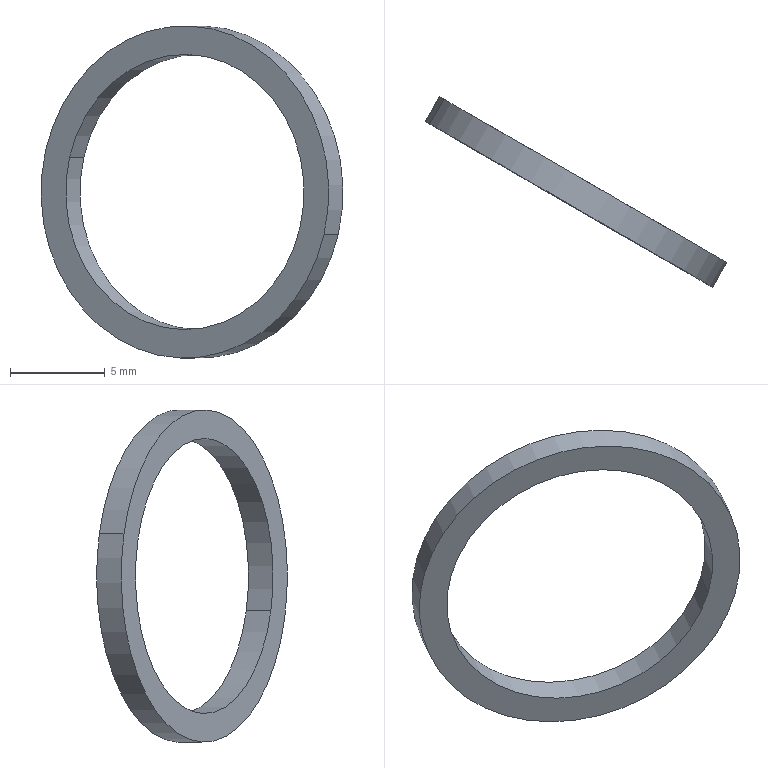Part | SolidWorks | features BaseBody 1 | 1 solid | 6 faces | box 15.905 x 10.049 x 17.5 mm | volume 113.097 mm3 | cylinder 4 | plane 2 | commonest cylinder face diameters 14.5 x2 17.5 x2
STEP:
#1=CARTESIAN_POINT('',(336.623,262.923,-1.84));
#2=VERTEX_POINT('',#1);
#3=CARTESIAN_POINT('',(324.477,269.935,1.84));
#4=VERTEX_POINT('',#3);
#5=CARTESIAN_POINT('',(330.55,266.429,0.));
#6=DIRECTION('',(0.5,0.866,0.));
#7=DIRECTION('',(-0.8377,0.4836,0.2538));
#8=AXIS2_PLACEMENT_3D('',#5,#6,#7);
#9=CIRCLE('',#8,7.25);
#10=EDGE_CURVE('',#2,#4,#9,.T.);
#11=ORIENTED_EDGE('',*,*,#10,.T.);
#12=CARTESIAN_POINT('',(323.727,268.636,1.84));
#13=VERTEX_POINT('',#12);
#14=CARTESIAN_POINT('',(324.477,269.935,1.84));
#15=DIRECTION('',(-0.5,-0.866,0.));
#16=VECTOR('',#15,1000.);
#17=LINE('',#14,#16);
#18=EDGE_CURVE('',#4,#13,#17,.T.);
#19=ORIENTED_EDGE('',*,*,#18,.T.);
#20=CARTESIAN_POINT('',(335.873,261.624,-1.84));
#21=VERTEX_POINT('',#20);
#22=CARTESIAN_POINT('',(329.8,265.13,0.));
#23=DIRECTION('',(0.5,0.866,0.));
#24=DIRECTION('',(-0.8377,0.4836,0.2538));
#25=AXIS2_PLACEMENT_3D('',#22,#23,#24);
#26=CIRCLE('',#25,7.25);
#27=EDGE_CURVE('',#21,#13,#26,.T.);
#28=ORIENTED_EDGE('',*,*,#27,.F.);
#29=CARTESIAN_POINT('',(336.623,262.923,-1.84));
#30=DIRECTION('',(-0.5,-0.866,0.));
#31=VECTOR('',#30,1000.);
#32=LINE('',#29,#31);
#33=EDGE_CURVE('',#2,#21,#32,.T.);
#34=ORIENTED_EDGE('',*,*,#33,.F.);
#35=EDGE_LOOP('',(#11,#19,#28,#34));
#36=FACE_OUTER_BOUND('',#35,.T.);
#37=CARTESIAN_POINT('',(330.55,266.429,0.));
#38=DIRECTION('',(-0.5,-0.866,0.));
#39=DIRECTION('',(0.8377,-0.4836,-0.2538));
#40=AXIS2_PLACEMENT_3D('',#37,#38,#39);
#41=CYLINDRICAL_SURFACE('',#40,7.25);
#42=ADVANCED_FACE('',(#36),#41,.F.);
#43=CARTESIAN_POINT('',(323.22,270.661,2.221));
#44=VERTEX_POINT('',#43);
#45=CARTESIAN_POINT('',(337.88,262.197,-2.221));
#46=VERTEX_POINT('',#45);
#47=CARTESIAN_POINT('',(330.55,266.429,0.));
#48=DIRECTION('',(0.5,0.866,0.));
#49=DIRECTION('',(-0.8377,0.4836,0.2538));
#50=AXIS2_PLACEMENT_3D('',#47,#48,#49);
#51=CIRCLE('',#50,8.75);
#52=EDGE_CURVE('',#44,#46,#51,.T.);
#53=ORIENTED_EDGE('',*,*,#52,.F.);
#54=CARTESIAN_POINT('',(322.47,269.362,2.221));
#55=VERTEX_POINT('',#54);
#56=CARTESIAN_POINT('',(323.22,270.661,2.221));
#57=DIRECTION('',(-0.5,-0.866,0.));
#58=VECTOR('',#57,1000.);
#59=LINE('',#56,#58);
#60=EDGE_CURVE('',#44,#55,#59,.T.);
#61=ORIENTED_EDGE('',*,*,#60,.T.);
#62=CARTESIAN_POINT('',(337.13,260.898,-2.221));
#63=VERTEX_POINT('',#62);
#64=CARTESIAN_POINT('',(329.8,265.13,0.));
#65=DIRECTION('',(0.5,0.866,0.));
#66=DIRECTION('',(-0.8377,0.4836,0.2538));
#67=AXIS2_PLACEMENT_3D('',#64,#65,#66);
#68=CIRCLE('',#67,8.75);
#69=EDGE_CURVE('',#55,#63,#68,.T.);
#70=ORIENTED_EDGE('',*,*,#69,.T.);
#71=CARTESIAN_POINT('',(337.88,262.197,-2.221));
#72=DIRECTION('',(-0.5,-0.866,0.));
#73=VECTOR('',#72,1000.);
#74=LINE('',#71,#73);
#75=EDGE_CURVE('',#46,#63,#74,.T.);
#76=ORIENTED_EDGE('',*,*,#75,.F.);
#77=EDGE_LOOP('',(#53,#61,#70,#76));
#78=FACE_OUTER_BOUND('',#77,.T.);
#79=CARTESIAN_POINT('',(330.55,266.429,0.));
#80=DIRECTION('',(-0.5,-0.866,0.));
#81=DIRECTION('',(0.8377,-0.4836,-0.2538));
#82=AXIS2_PLACEMENT_3D('',#79,#80,#81);
#83=CYLINDRICAL_SURFACE('',#82,8.75);
#84=ADVANCED_FACE('',(#78),#83,.T.);
#85=CARTESIAN_POINT('',(330.55,266.429,0.));
#86=DIRECTION('',(0.5,0.866,0.));
#87=DIRECTION('',(-0.8377,0.4836,0.2538));
#88=AXIS2_PLACEMENT_3D('',#85,#86,#87);
#89=CIRCLE('',#88,8.75);
#90=EDGE_CURVE('',#46,#44,#89,.T.);
#91=ORIENTED_EDGE('',*,*,#90,.T.);
#92=ORIENTED_EDGE('',*,*,#52,.T.);
#93=EDGE_LOOP('',(#91,#92));
#94=FACE_OUTER_BOUND('',#93,.T.);
#95=ORIENTED_EDGE('',*,*,#10,.F.);
#96=CARTESIAN_POINT('',(330.55,266.429,0.));
#97=DIRECTION('',(0.5,0.866,0.));
#98=DIRECTION('',(-0.8377,0.4836,0.2538));
#99=AXIS2_PLACEMENT_3D('',#96,#97,#98);
#100=CIRCLE('',#99,7.25);
#101=EDGE_CURVE('',#4,#2,#100,.T.);
#102=ORIENTED_EDGE('',*,*,#101,.F.);
#103=EDGE_LOOP('',(#95,#102));
#104=FACE_BOUND('',#103,.T.);
#105=CARTESIAN_POINT('',(330.55,266.429,0.));
#106=DIRECTION('',(0.5,0.866,0.));
#107=DIRECTION('',(-0.8377,0.4836,0.2538));
#108=AXIS2_PLACEMENT_3D('',#105,#106,#107);
#109=PLANE('',#108);
#110=ADVANCED_FACE('',(#94,#104),#109,.T.);
#111=CARTESIAN_POINT('',(329.8,265.13,0.));
#112=DIRECTION('',(0.5,0.866,0.));
#113=DIRECTION('',(-0.8377,0.4836,0.2538));
#114=AXIS2_PLACEMENT_3D('',#111,#112,#113);
#115=CIRCLE('',#114,8.75);
#116=EDGE_CURVE('',#63,#55,#115,.T.);
#117=ORIENTED_EDGE('',*,*,#116,.F.);
#118=ORIENTED_EDGE('',*,*,#69,.F.);
#119=EDGE_LOOP('',(#117,#118));
#120=FACE_OUTER_BOUND('',#119,.T.);
#121=ORIENTED_EDGE('',*,*,#27,.T.);
#122=CARTESIAN_POINT('',(329.8,265.13,0.));
#123=DIRECTION('',(0.5,0.866,0.));
#124=DIRECTION('',(-0.8377,0.4836,0.2538));
#125=AXIS2_PLACEMENT_3D('',#122,#123,#124);
#126=CIRCLE('',#125,7.25);
#127=EDGE_CURVE('',#13,#21,#126,.T.);
#128=ORIENTED_EDGE('',*,*,#127,.T.);
#129=EDGE_LOOP('',(#121,#128));
#130=FACE_BOUND('',#129,.T.);
#131=CARTESIAN_POINT('',(329.8,265.13,0.));
#132=DIRECTION('',(0.5,0.866,0.));
#133=DIRECTION('',(-0.8377,0.4836,0.2538));
#134=AXIS2_PLACEMENT_3D('',#131,#132,#133);
#135=PLANE('',#134);
#136=ADVANCED_FACE('',(#120,#130),#135,.F.);
#137=ORIENTED_EDGE('',*,*,#60,.F.);
#138=ORIENTED_EDGE('',*,*,#90,.F.);
#139=ORIENTED_EDGE('',*,*,#75,.T.);
#140=ORIENTED_EDGE('',*,*,#116,.T.);
#141=EDGE_LOOP('',(#137,#138,#139,#140));
#142=FACE_OUTER_BOUND('',#141,.T.);
#143=CARTESIAN_POINT('',(330.55,266.429,0.));
#144=DIRECTION('',(-0.5,-0.866,0.));
#145=DIRECTION('',(0.8377,-0.4836,-0.2538));
#146=AXIS2_PLACEMENT_3D('',#143,#144,#145);
#147=CYLINDRICAL_SURFACE('',#146,8.75);
#148=ADVANCED_FACE('',(#142),#147,.T.);
#149=ORIENTED_EDGE('',*,*,#18,.F.);
#150=ORIENTED_EDGE('',*,*,#101,.T.);
#151=ORIENTED_EDGE('',*,*,#33,.T.);
#152=ORIENTED_EDGE('',*,*,#127,.F.);
#153=EDGE_LOOP('',(#149,#150,#151,#152));
#154=FACE_OUTER_BOUND('',#153,.T.);
#155=CARTESIAN_POINT('',(330.55,266.429,0.));
#156=DIRECTION('',(-0.5,-0.866,0.));
#157=DIRECTION('',(0.8377,-0.4836,-0.2538));
#158=AXIS2_PLACEMENT_3D('',#155,#156,#157);
#159=CYLINDRICAL_SURFACE('',#158,7.25);
#160=ADVANCED_FACE('',(#154),#159,.F.);
#161=CLOSED_SHELL('',(#42,#84,#110,#136,#148,#160));
#162=MANIFOLD_SOLID_BREP('',#161);
#163=CARTESIAN_POINT('',(0.,0.,0.));
#164=DIRECTION('',(0.,0.,1.));
#165=DIRECTION('',(1.,0.,0.));
#166=AXIS2_PLACEMENT_3D('',#163,#164,#165);
#167=(LENGTH_UNIT()NAMED_UNIT(*)SI_UNIT(.MILLI.,.METRE.));
#168=UNCERTAINTY_MEASURE_WITH_UNIT(LENGTH_MEASURE(0.00001),#167,'','');
#169=(NAMED_UNIT(*)PLANE_ANGLE_UNIT()SI_UNIT($,.RADIAN.));
#170=(NAMED_UNIT(*)SI_UNIT($,.STERADIAN.)SOLID_ANGLE_UNIT());
#171=(GEOMETRIC_REPRESENTATION_CONTEXT(3)GLOBAL_UNCERTAINTY_ASSIGNED_CONTEXT((#168))GLOBAL_UNIT_ASSIGNED_CONTEXT((#167,#169,#170))REPRESENTATION_CONTEXT('',''));
#172=ADVANCED_BREP_SHAPE_REPRESENTATION('',(#162,#166),#171);